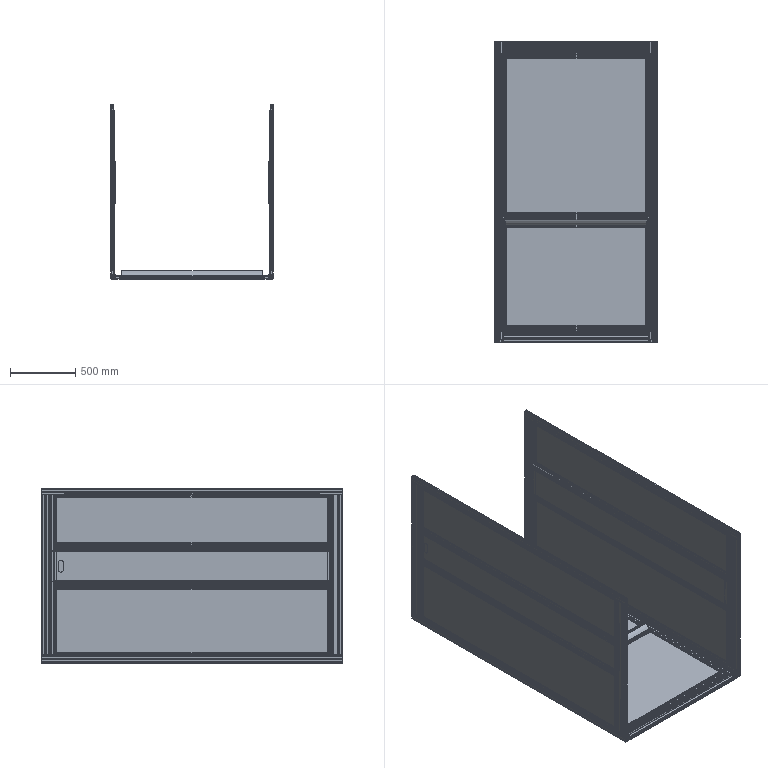Part | SolidWorks | features ReferencePattern 10, MirrorCompFeat 5 | 144 solids | 5046 faces | volume 235752784 mm3 | plane 3284 | cylinder 1762 | commonest cylinder face diameters 1.1 x216 8.5 x204 3.6 x184 5.8 x178 0.4 x124 0.6 x112